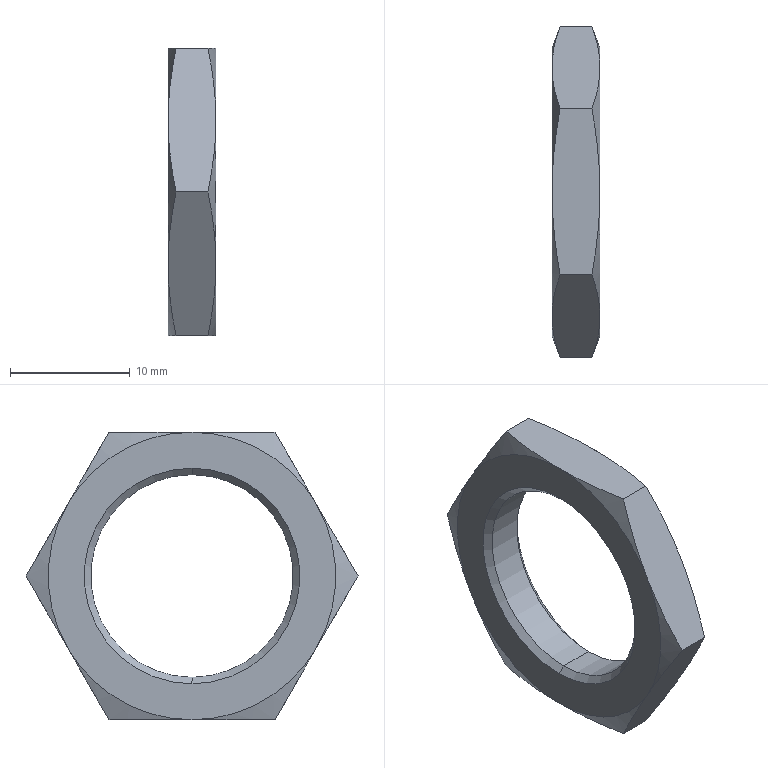Part | SolidWorks | features BaseBody 1 | 1 solid | 26 faces | box 4 x 27.713 x 24 mm | volume 1061 mm3 | cone 16 | plane 8 | cylinder 2 | commonest cylinder face diameters 16.917 x2
STEP:
#1=CARTESIAN_POINT('',(1.458,0.,8.459));
#2=VERTEX_POINT('',#1);
#3=CARTESIAN_POINT('',(1.458,0.,-8.459));
#4=VERTEX_POINT('',#3);
#5=CARTESIAN_POINT('',(1.458,0.,0.));
#6=DIRECTION('',(1.,0.,0.));
#7=DIRECTION('',(0.,0.,-1.));
#8=AXIS2_PLACEMENT_3D('',#5,#6,#7);
#9=CIRCLE('',#8,8.459);
#10=EDGE_CURVE('',#2,#4,#9,.T.);
#11=ORIENTED_EDGE('',*,*,#10,.F.);
#12=CARTESIAN_POINT('',(2.,0.,9.));
#13=VERTEX_POINT('',#12);
#14=CARTESIAN_POINT('',(2.,0.,9.));
#15=DIRECTION('',(0.7071,0.,0.7071));
#16=VECTOR('',#15,1000.);
#17=LINE('',#14,#16);
#18=EDGE_CURVE('',#2,#13,#17,.T.);
#19=ORIENTED_EDGE('',*,*,#18,.T.);
#20=CARTESIAN_POINT('',(2.,0.,-9.));
#21=VERTEX_POINT('',#20);
#22=CARTESIAN_POINT('',(2.,0.,0.));
#23=DIRECTION('',(1.,0.,0.));
#24=DIRECTION('',(0.,0.,-1.));
#25=AXIS2_PLACEMENT_3D('',#22,#23,#24);
#26=CIRCLE('',#25,9.);
#27=EDGE_CURVE('',#13,#21,#26,.T.);
#28=ORIENTED_EDGE('',*,*,#27,.T.);
#29=CARTESIAN_POINT('',(2.,0.,-9.));
#30=DIRECTION('',(0.7071,0.,-0.7071));
#31=VECTOR('',#30,1000.);
#32=LINE('',#29,#31);
#33=EDGE_CURVE('',#4,#21,#32,.T.);
#34=ORIENTED_EDGE('',*,*,#33,.F.);
#35=EDGE_LOOP('',(#11,#19,#28,#34));
#36=FACE_OUTER_BOUND('',#35,.T.);
#37=CARTESIAN_POINT('',(2.,0.,0.));
#38=DIRECTION('',(1.,0.,0.));
#39=DIRECTION('',(0.,0.,-1.));
#40=AXIS2_PLACEMENT_3D('',#37,#38,#39);
#41=CONICAL_SURFACE('',#40,9.,0.7854);
#42=ADVANCED_FACE('',(#36),#41,.F.);
#43=ORIENTED_EDGE('',*,*,#10,.T.);
#44=CARTESIAN_POINT('',(-1.458,0.,-8.459));
#45=VERTEX_POINT('',#44);
#46=CARTESIAN_POINT('',(2.,0.,-8.459));
#47=DIRECTION('',(-1.,0.,0.));
#48=VECTOR('',#47,1000.);
#49=LINE('',#46,#48);
#50=EDGE_CURVE('',#4,#45,#49,.T.);
#51=ORIENTED_EDGE('',*,*,#50,.T.);
#52=CARTESIAN_POINT('',(-1.458,0.,8.459));
#53=VERTEX_POINT('',#52);
#54=CARTESIAN_POINT('',(-1.458,0.,0.));
#55=DIRECTION('',(1.,0.,0.));
#56=DIRECTION('',(0.,0.,1.));
#57=AXIS2_PLACEMENT_3D('',#54,#55,#56);
#58=CIRCLE('',#57,8.459);
#59=EDGE_CURVE('',#53,#45,#58,.T.);
#60=ORIENTED_EDGE('',*,*,#59,.F.);
#61=CARTESIAN_POINT('',(2.,0.,8.459));
#62=DIRECTION('',(-1.,0.,0.));
#63=VECTOR('',#62,1000.);
#64=LINE('',#61,#63);
#65=EDGE_CURVE('',#2,#53,#64,.T.);
#66=ORIENTED_EDGE('',*,*,#65,.F.);
#67=EDGE_LOOP('',(#43,#51,#60,#66));
#68=FACE_OUTER_BOUND('',#67,.T.);
#69=CARTESIAN_POINT('',(2.,0.,0.));
#70=DIRECTION('',(-1.,0.,0.));
#71=DIRECTION('',(0.,0.,1.));
#72=AXIS2_PLACEMENT_3D('',#69,#70,#71);
#73=CYLINDRICAL_SURFACE('',#72,8.459);
#74=ADVANCED_FACE('',(#68),#73,.F.);
#75=ORIENTED_EDGE('',*,*,#59,.T.);
#76=CARTESIAN_POINT('',(-2.,0.,-9.));
#77=VERTEX_POINT('',#76);
#78=CARTESIAN_POINT('',(-2.,0.,-9.));
#79=DIRECTION('',(-0.7071,0.,-0.7071));
#80=VECTOR('',#79,1000.);
#81=LINE('',#78,#80);
#82=EDGE_CURVE('',#45,#77,#81,.T.);
#83=ORIENTED_EDGE('',*,*,#82,.T.);
#84=CARTESIAN_POINT('',(-2.,0.,9.));
#85=VERTEX_POINT('',#84);
#86=CARTESIAN_POINT('',(-2.,0.,0.));
#87=DIRECTION('',(1.,0.,0.));
#88=DIRECTION('',(0.,0.,1.));
#89=AXIS2_PLACEMENT_3D('',#86,#87,#88);
#90=CIRCLE('',#89,9.);
#91=EDGE_CURVE('',#85,#77,#90,.T.);
#92=ORIENTED_EDGE('',*,*,#91,.F.);
#93=CARTESIAN_POINT('',(-2.,0.,9.));
#94=DIRECTION('',(-0.7071,0.,0.7071));
#95=VECTOR('',#94,1000.);
#96=LINE('',#93,#95);
#97=EDGE_CURVE('',#53,#85,#96,.T.);
#98=ORIENTED_EDGE('',*,*,#97,.F.);
#99=EDGE_LOOP('',(#75,#83,#92,#98));
#100=FACE_OUTER_BOUND('',#99,.T.);
#101=CARTESIAN_POINT('',(-2.,0.,0.));
#102=DIRECTION('',(-1.,0.,0.));
#103=DIRECTION('',(0.,0.,1.));
#104=AXIS2_PLACEMENT_3D('',#101,#102,#103);
#105=CONICAL_SURFACE('',#104,9.,0.7854);
#106=ADVANCED_FACE('',(#100),#105,.F.);
#107=CARTESIAN_POINT('',(2.,10.392,6.));
#108=VERTEX_POINT('',#107);
#109=CARTESIAN_POINT('',(2.,10.392,-6.));
#110=VERTEX_POINT('',#109);
#111=CARTESIAN_POINT('',(2.,0.,0.));
#112=DIRECTION('',(-1.,0.,0.));
#113=DIRECTION('',(0.,0.,1.));
#114=AXIS2_PLACEMENT_3D('',#111,#112,#113);
#115=CIRCLE('',#114,12.);
#116=EDGE_CURVE('',#108,#110,#115,.T.);
#117=ORIENTED_EDGE('',*,*,#116,.F.);
#118=CARTESIAN_POINT('',(2.,0.,12.));
#119=VERTEX_POINT('',#118);
#120=CARTESIAN_POINT('',(2.,0.,0.));
#121=DIRECTION('',(-1.,0.,0.));
#122=DIRECTION('',(0.,0.,1.));
#123=AXIS2_PLACEMENT_3D('',#120,#121,#122);
#124=CIRCLE('',#123,12.);
#125=EDGE_CURVE('',#119,#108,#124,.T.);
#126=ORIENTED_EDGE('',*,*,#125,.F.);
#127=CARTESIAN_POINT('',(2.,-10.392,6.));
#128=VERTEX_POINT('',#127);
#129=CARTESIAN_POINT('',(2.,0.,0.));
#130=DIRECTION('',(-1.,0.,0.));
#131=DIRECTION('',(0.,0.,1.));
#132=AXIS2_PLACEMENT_3D('',#129,#130,#131);
#133=CIRCLE('',#132,12.);
#134=EDGE_CURVE('',#128,#119,#133,.T.);
#135=ORIENTED_EDGE('',*,*,#134,.F.);
#136=CARTESIAN_POINT('',(2.,-10.392,-6.));
#137=VERTEX_POINT('',#136);
#138=CARTESIAN_POINT('',(2.,0.,0.));
#139=DIRECTION('',(-1.,0.,0.));
#140=DIRECTION('',(0.,0.,1.));
#141=AXIS2_PLACEMENT_3D('',#138,#139,#140);
#142=CIRCLE('',#141,12.);
#143=EDGE_CURVE('',#137,#128,#142,.T.);
#144=ORIENTED_EDGE('',*,*,#143,.F.);
#145=CARTESIAN_POINT('',(2.,0.,-12.));
#146=VERTEX_POINT('',#145);
#147=CARTESIAN_POINT('',(2.,0.,0.));
#148=DIRECTION('',(-1.,0.,0.));
#149=DIRECTION('',(0.,0.,1.));
#150=AXIS2_PLACEMENT_3D('',#147,#148,#149);
#151=CIRCLE('',#150,12.);
#152=EDGE_CURVE('',#146,#137,#151,.T.);
#153=ORIENTED_EDGE('',*,*,#152,.F.);
#154=CARTESIAN_POINT('',(2.,0.,0.));
#155=DIRECTION('',(-1.,0.,0.));
#156=DIRECTION('',(0.,0.,1.));
#157=AXIS2_PLACEMENT_3D('',#154,#155,#156);
#158=CIRCLE('',#157,12.);
#159=EDGE_CURVE('',#110,#146,#158,.T.);
#160=ORIENTED_EDGE('',*,*,#159,.F.);
#161=EDGE_LOOP('',(#117,#126,#135,#144,#153,#160));
#162=FACE_OUTER_BOUND('',#161,.T.);
#163=CARTESIAN_POINT('',(2.,0.,0.));
#164=DIRECTION('',(1.,0.,0.));
#165=DIRECTION('',(0.,0.,-1.));
#166=AXIS2_PLACEMENT_3D('',#163,#164,#165);
#167=CIRCLE('',#166,9.);
#168=EDGE_CURVE('',#21,#13,#167,.T.);
#169=ORIENTED_EDGE('',*,*,#168,.F.);
#170=ORIENTED_EDGE('',*,*,#27,.F.);
#171=EDGE_LOOP('',(#169,#170));
#172=FACE_BOUND('',#171,.T.);
#173=CARTESIAN_POINT('',(2.,12.,0.));
#174=DIRECTION('',(-1.,0.,0.));
#175=DIRECTION('',(0.,0.,1.));
#176=AXIS2_PLACEMENT_3D('',#173,#174,#175);
#177=PLANE('',#176);
#178=ADVANCED_FACE('',(#162,#172),#177,.F.);
#179=CARTESIAN_POINT('',(1.324,6.928,-12.));
#180=VERTEX_POINT('',#179);
#181=CARTESIAN_POINT('',(1.324,6.928,-12.));
#182=CARTESIAN_POINT('',(1.533,7.501,-11.008));
#183=CARTESIAN_POINT('',(1.703,8.075,-10.013));
#184=CARTESIAN_POINT('',(1.937,9.23,-8.014));
#185=CARTESIAN_POINT('',(2.,9.809,-7.01));
#186=CARTESIAN_POINT('',(2.,10.392,-6.));
#187=B_SPLINE_CURVE_WITH_KNOTS('',3,(#181,#182,#183,#184,#185,#186),.UNSPECIFIED.,.F.,.F.,(4,2,4),(0.,0.003481,0.006961),.UNSPECIFIED.);
#188=EDGE_CURVE('',#180,#110,#187,.T.);
#189=ORIENTED_EDGE('',*,*,#188,.T.);
#190=ORIENTED_EDGE('',*,*,#159,.T.);
#191=CARTESIAN_POINT('',(2.,0.,-12.));
#192=CARTESIAN_POINT('',(2.,1.166,-12.));
#193=CARTESIAN_POINT('',(1.937,2.325,-12.));
#194=CARTESIAN_POINT('',(1.703,4.634,-12.));
#195=CARTESIAN_POINT('',(1.533,5.783,-12.));
#196=CARTESIAN_POINT('',(1.324,6.928,-12.));
#197=B_SPLINE_CURVE_WITH_KNOTS('',3,(#191,#192,#193,#194,#195,#196),.UNSPECIFIED.,.F.,.F.,(4,2,4),(0.,0.003481,0.006961),.UNSPECIFIED.);
#198=EDGE_CURVE('',#146,#180,#197,.T.);
#199=ORIENTED_EDGE('',*,*,#198,.T.);
#200=EDGE_LOOP('',(#189,#190,#199));
#201=FACE_OUTER_BOUND('',#200,.T.);
#202=CARTESIAN_POINT('',(1.32,0.,0.));
#203=DIRECTION('',(-1.,0.,0.));
#204=DIRECTION('',(0.,0.,1.));
#205=AXIS2_PLACEMENT_3D('',#202,#203,#204);
#206=CONICAL_SURFACE('',#205,13.868,1.222);
#207=ADVANCED_FACE('',(#201),#206,.T.);
#208=CARTESIAN_POINT('',(1.324,13.856,-0.000000041));
#209=VERTEX_POINT('',#208);
#210=CARTESIAN_POINT('',(2.,10.392,-6.));
#211=CARTESIAN_POINT('',(2.,10.975,-4.99));
#212=CARTESIAN_POINT('',(1.937,11.555,-3.986));
#213=CARTESIAN_POINT('',(1.703,12.709,-1.987));
#214=CARTESIAN_POINT('',(1.533,13.284,-0.9919));
#215=CARTESIAN_POINT('',(1.324,13.856,-0.000000041));
#216=B_SPLINE_CURVE_WITH_KNOTS('',3,(#210,#211,#212,#213,#214,#215),.UNSPECIFIED.,.F.,.F.,(4,2,4),(0.,0.003481,0.006961),.UNSPECIFIED.);
#217=EDGE_CURVE('',#110,#209,#216,.T.);
#218=ORIENTED_EDGE('',*,*,#217,.T.);
#219=CARTESIAN_POINT('',(1.324,13.856,-0.000000041));
#220=CARTESIAN_POINT('',(1.533,13.284,0.9919));
#221=CARTESIAN_POINT('',(1.703,12.709,1.987));
#222=CARTESIAN_POINT('',(1.937,11.555,3.986));
#223=CARTESIAN_POINT('',(2.,10.975,4.99));
#224=CARTESIAN_POINT('',(2.,10.392,6.));
#225=B_SPLINE_CURVE_WITH_KNOTS('',3,(#219,#220,#221,#222,#223,#224),.UNSPECIFIED.,.F.,.F.,(4,2,4),(0.,0.003481,0.006961),.UNSPECIFIED.);
#226=EDGE_CURVE('',#209,#108,#225,.T.);
#227=ORIENTED_EDGE('',*,*,#226,.T.);
#228=ORIENTED_EDGE('',*,*,#116,.T.);
#229=EDGE_LOOP('',(#218,#227,#228));
#230=FACE_OUTER_BOUND('',#229,.T.);
#231=CARTESIAN_POINT('',(1.32,0.,0.));
#232=DIRECTION('',(-1.,0.,0.));
#233=DIRECTION('',(0.,0.,1.));
#234=AXIS2_PLACEMENT_3D('',#231,#232,#233);
#235=CONICAL_SURFACE('',#234,13.868,1.222);
#236=ADVANCED_FACE('',(#230),#235,.T.);
#237=CARTESIAN_POINT('',(1.324,6.928,12.));
#238=VERTEX_POINT('',#237);
#239=CARTESIAN_POINT('',(2.,10.392,6.));
#240=CARTESIAN_POINT('',(2.,9.809,7.01));
#241=CARTESIAN_POINT('',(1.937,9.23,8.014));
#242=CARTESIAN_POINT('',(1.703,8.075,10.013));
#243=CARTESIAN_POINT('',(1.533,7.501,11.008));
#244=CARTESIAN_POINT('',(1.324,6.928,12.));
#245=B_SPLINE_CURVE_WITH_KNOTS('',3,(#239,#240,#241,#242,#243,#244),.UNSPECIFIED.,.F.,.F.,(4,2,4),(0.,0.003481,0.006961),.UNSPECIFIED.);
#246=EDGE_CURVE('',#108,#238,#245,.T.);
#247=ORIENTED_EDGE('',*,*,#246,.T.);
#248=CARTESIAN_POINT('',(1.324,6.928,12.));
#249=CARTESIAN_POINT('',(1.533,5.783,12.));
#250=CARTESIAN_POINT('',(1.703,4.634,12.));
#251=CARTESIAN_POINT('',(1.937,2.325,12.));
#252=CARTESIAN_POINT('',(2.,1.166,12.));
#253=CARTESIAN_POINT('',(2.,0.,12.));
#254=B_SPLINE_CURVE_WITH_KNOTS('',3,(#248,#249,#250,#251,#252,#253),.UNSPECIFIED.,.F.,.F.,(4,2,4),(0.,0.003481,0.006961),.UNSPECIFIED.);
#255=EDGE_CURVE('',#238,#119,#254,.T.);
#256=ORIENTED_EDGE('',*,*,#255,.T.);
#257=ORIENTED_EDGE('',*,*,#125,.T.);
#258=EDGE_LOOP('',(#247,#256,#257));
#259=FACE_OUTER_BOUND('',#258,.T.);
#260=CARTESIAN_POINT('',(1.32,0.,0.));
#261=DIRECTION('',(-1.,0.,0.));
#262=DIRECTION('',(0.,0.,1.));
#263=AXIS2_PLACEMENT_3D('',#260,#261,#262);
#264=CONICAL_SURFACE('',#263,13.868,1.222);
#265=ADVANCED_FACE('',(#259),#264,.T.);
#266=CARTESIAN_POINT('',(1.324,-6.928,12.));
#267=VERTEX_POINT('',#266);
#268=CARTESIAN_POINT('',(2.,0.,12.));
#269=CARTESIAN_POINT('',(2.,-1.166,12.));
#270=CARTESIAN_POINT('',(1.937,-2.325,12.));
#271=CARTESIAN_POINT('',(1.703,-4.634,12.));
#272=CARTESIAN_POINT('',(1.533,-5.783,12.));
#273=CARTESIAN_POINT('',(1.324,-6.928,12.));
#274=B_SPLINE_CURVE_WITH_KNOTS('',3,(#268,#269,#270,#271,#272,#273),.UNSPECIFIED.,.F.,.F.,(4,2,4),(0.,0.003481,0.006961),.UNSPECIFIED.);
#275=EDGE_CURVE('',#119,#267,#274,.T.);
#276=ORIENTED_EDGE('',*,*,#275,.T.);
#277=CARTESIAN_POINT('',(1.324,-6.928,12.));
#278=CARTESIAN_POINT('',(1.533,-7.501,11.008));
#279=CARTESIAN_POINT('',(1.703,-8.075,10.013));
#280=CARTESIAN_POINT('',(1.937,-9.23,8.014));
#281=CARTESIAN_POINT('',(2.,-9.809,7.01));
#282=CARTESIAN_POINT('',(2.,-10.392,6.));
#283=B_SPLINE_CURVE_WITH_KNOTS('',3,(#277,#278,#279,#280,#281,#282),.UNSPECIFIED.,.F.,.F.,(4,2,4),(0.,0.003481,0.006961),.UNSPECIFIED.);
#284=EDGE_CURVE('',#267,#128,#283,.T.);
#285=ORIENTED_EDGE('',*,*,#284,.T.);
#286=ORIENTED_EDGE('',*,*,#134,.T.);
#287=EDGE_LOOP('',(#276,#285,#286));
#288=FACE_OUTER_BOUND('',#287,.T.);
#289=CARTESIAN_POINT('',(1.32,0.,0.));
#290=DIRECTION('',(-1.,0.,0.));
#291=DIRECTION('',(0.,0.,1.));
#292=AXIS2_PLACEMENT_3D('',#289,#290,#291);
#293=CONICAL_SURFACE('',#292,13.868,1.222);
#294=ADVANCED_FACE('',(#288),#293,.T.);
#295=CARTESIAN_POINT('',(1.324,-13.856,0.000000041));
#296=VERTEX_POINT('',#295);
#297=CARTESIAN_POINT('',(1.324,-13.856,0.000000041));
#298=CARTESIAN_POINT('',(1.533,-13.284,-0.9919));
#299=CARTESIAN_POINT('',(1.703,-12.709,-1.987));
#300=CARTESIAN_POINT('',(1.937,-11.555,-3.986));
#301=CARTESIAN_POINT('',(2.,-10.975,-4.99));
#302=CARTESIAN_POINT('',(2.,-10.392,-6.));
#303=B_SPLINE_CURVE_WITH_KNOTS('',3,(#297,#298,#299,#300,#301,#302),.UNSPECIFIED.,.F.,.F.,(4,2,4),(0.,0.003481,0.006961),.UNSPECIFIED.);
#304=EDGE_CURVE('',#296,#137,#303,.T.);
#305=ORIENTED_EDGE('',*,*,#304,.T.);
#306=ORIENTED_EDGE('',*,*,#143,.T.);
#307=CARTESIAN_POINT('',(2.,-10.392,6.));
#308=CARTESIAN_POINT('',(2.,-10.975,4.99));
#309=CARTESIAN_POINT('',(1.937,-11.555,3.986));
#310=CARTESIAN_POINT('',(1.703,-12.709,1.987));
#311=CARTESIAN_POINT('',(1.533,-13.284,0.9919));
#312=CARTESIAN_POINT('',(1.324,-13.856,0.000000041));
#313=B_SPLINE_CURVE_WITH_KNOTS('',3,(#307,#308,#309,#310,#311,#312),.UNSPECIFIED.,.F.,.F.,(4,2,4),(0.,0.003481,0.006961),.UNSPECIFIED.);
#314=EDGE_CURVE('',#128,#296,#313,.T.);
#315=ORIENTED_EDGE('',*,*,#314,.T.);
#316=EDGE_LOOP('',(#305,#306,#315));
#317=FACE_OUTER_BOUND('',#316,.T.);
#318=CARTESIAN_POINT('',(1.32,0.,0.));
#319=DIRECTION('',(-1.,0.,0.));
#320=DIRECTION('',(0.,0.,1.));
#321=AXIS2_PLACEMENT_3D('',#318,#319,#320);
#322=CONICAL_SURFACE('',#321,13.868,1.222);
#323=ADVANCED_FACE('',(#317),#322,.T.);
#324=CARTESIAN_POINT('',(1.324,-6.928,-12.));
#325=VERTEX_POINT('',#324);
#326=CARTESIAN_POINT('',(1.324,-6.928,-12.));
#327=CARTESIAN_POINT('',(1.533,-5.783,-12.));
#328=CARTESIAN_POINT('',(1.703,-4.634,-12.));
#329=CARTESIAN_POINT('',(1.937,-2.325,-12.));
#330=CARTESIAN_POINT('',(2.,-1.166,-12.));
#331=CARTESIAN_POINT('',(2.,0.,-12.));
#332=B_SPLINE_CURVE_WITH_KNOTS('',3,(#326,#327,#328,#329,#330,#331),.UNSPECIFIED.,.F.,.F.,(4,2,4),(0.,0.003481,0.006961),.UNSPECIFIED.);
#333=EDGE_CURVE('',#325,#146,#332,.T.);
#334=ORIENTED_EDGE('',*,*,#333,.T.);
#335=ORIENTED_EDGE('',*,*,#152,.T.);
#336=CARTESIAN_POINT('',(2.,-10.392,-6.));
#337=CARTESIAN_POINT('',(2.,-9.809,-7.01));
#338=CARTESIAN_POINT('',(1.937,-9.23,-8.014));
#339=CARTESIAN_POINT('',(1.703,-8.075,-10.013));
#340=CARTESIAN_POINT('',(1.533,-7.501,-11.008));
#341=CARTESIAN_POINT('',(1.324,-6.928,-12.));
#342=B_SPLINE_CURVE_WITH_KNOTS('',3,(#336,#337,#338,#339,#340,#341),.UNSPECIFIED.,.F.,.F.,(4,2,4),(0.,0.003481,0.006961),.UNSPECIFIED.);
#343=EDGE_CURVE('',#137,#325,#342,.T.);
#344=ORIENTED_EDGE('',*,*,#343,.T.);
#345=EDGE_LOOP('',(#334,#335,#344));
#346=FACE_OUTER_BOUND('',#345,.T.);
#347=CARTESIAN_POINT('',(1.32,0.,0.));
#348=DIRECTION('',(-1.,0.,0.));
#349=DIRECTION('',(0.,0.,1.));
#350=AXIS2_PLACEMENT_3D('',#347,#348,#349);
#351=CONICAL_SURFACE('',#350,13.868,1.222);
#352=ADVANCED_FACE('',(#346),#351,.T.);
#353=ORIENTED_EDGE('',*,*,#18,.F.);
#354=CARTESIAN_POINT('',(1.458,0.,0.));
#355=DIRECTION('',(1.,0.,0.));
#356=DIRECTION('',(0.,0.,-1.));
#357=AXIS2_PLACEMENT_3D('',#354,#355,#356);
#358=CIRCLE('',#357,8.459);
#359=EDGE_CURVE('',#4,#2,#358,.T.);
#360=ORIENTED_EDGE('',*,*,#359,.F.);
#361=ORIENTED_EDGE('',*,*,#33,.T.);
#362=ORIENTED_EDGE('',*,*,#168,.T.);
#363=EDGE_LOOP('',(#353,#360,#361,#362));
#364=FACE_OUTER_BOUND('',#363,.T.);
#365=CARTESIAN_POINT('',(2.,0.,0.));
#366=DIRECTION('',(1.,0.,0.));
#367=DIRECTION('',(0.,0.,-1.));
#368=AXIS2_PLACEMENT_3D('',#365,#366,#367);
#369=CONICAL_SURFACE('',#368,9.,0.7854);
#370=ADVANCED_FACE('',(#364),#369,.F.);
#371=ORIENTED_EDGE('',*,*,#217,.F.);
#372=ORIENTED_EDGE('',*,*,#188,.F.);
#373=CARTESIAN_POINT('',(-1.324,6.928,-12.));
#374=VERTEX_POINT('',#373);
#375=CARTESIAN_POINT('',(4.,6.928,-12.));
#376=DIRECTION('',(1.,0.,0.));
#377=VECTOR('',#376,1000.);
#378=LINE('',#375,#377);
#379=EDGE_CURVE('',#374,#180,#378,.T.);
#380=ORIENTED_EDGE('',*,*,#379,.F.);
#381=CARTESIAN_POINT('',(-2.,10.392,-6.));
#382=VERTEX_POINT('',#381);
#383=CARTESIAN_POINT('',(-2.,10.392,-6.));
#384=CARTESIAN_POINT('',(-2.,9.809,-7.01));
#385=CARTESIAN_POINT('',(-1.937,9.23,-8.014));
#386=CARTESIAN_POINT('',(-1.703,8.075,-10.013));
#387=CARTESIAN_POINT('',(-1.533,7.501,-11.008));
#388=CARTESIAN_POINT('',(-1.324,6.928,-12.));
#389=B_SPLINE_CURVE_WITH_KNOTS('',3,(#383,#384,#385,#386,#387,#388),.UNSPECIFIED.,.F.,.F.,(4,2,4),(0.,0.003481,0.006961),.UNSPECIFIED.);
#390=EDGE_CURVE('',#382,#374,#389,.T.);
#391=ORIENTED_EDGE('',*,*,#390,.F.);
#392=CARTESIAN_POINT('',(-1.324,13.856,0.));
#393=VERTEX_POINT('',#392);
#394=CARTESIAN_POINT('',(-1.324,13.856,0.));
#395=CARTESIAN_POINT('',(-1.533,13.284,-0.9919));
#396=CARTESIAN_POINT('',(-1.703,12.709,-1.987));
#397=CARTESIAN_POINT('',(-1.937,11.555,-3.986));
#398=CARTESIAN_POINT('',(-2.,10.975,-4.99));
#399=CARTESIAN_POINT('',(-2.,10.392,-6.));
#400=B_SPLINE_CURVE_WITH_KNOTS('',3,(#394,#395,#396,#397,#398,#399),.UNSPECIFIED.,.F.,.F.,(4,2,4),(0.,0.003481,0.006961),.UNSPECIFIED.);
#401=EDGE_CURVE('',#393,#382,#400,.T.);
#402=ORIENTED_EDGE('',*,*,#401,.F.);
#403=CARTESIAN_POINT('',(4.,13.856,0.));
#404=DIRECTION('',(-1.,0.,0.));
#405=VECTOR('',#404,1000.);
#406=LINE('',#403,#405);
#407=EDGE_CURVE('',#209,#393,#406,.T.);
#408=ORIENTED_EDGE('',*,*,#407,.F.);
#409=EDGE_LOOP('',(#371,#372,#380,#391,#402,#408));
#410=FACE_OUTER_BOUND('',#409,.T.);
#411=CARTESIAN_POINT('',(4.,6.928,-12.));
#412=DIRECTION('',(0.,-0.866,0.5));
#413=DIRECTION('',(0.,-0.5,-0.866));
#414=AXIS2_PLACEMENT_3D('',#411,#412,#413);
#415=PLANE('',#414);
#416=ADVANCED_FACE('',(#410),#415,.F.);
#417=ORIENTED_EDGE('',*,*,#198,.F.);
#418=ORIENTED_EDGE('',*,*,#333,.F.);
#419=CARTESIAN_POINT('',(-1.324,-6.928,-12.));
#420=VERTEX_POINT('',#419);
#421=CARTESIAN_POINT('',(4.,-6.928,-12.));
#422=DIRECTION('',(1.,0.,0.));
#423=VECTOR('',#422,1000.);
#424=LINE('',#421,#423);
#425=EDGE_CURVE('',#420,#325,#424,.T.);
#426=ORIENTED_EDGE('',*,*,#425,.F.);
#427=CARTESIAN_POINT('',(-2.,0.,-12.));
#428=VERTEX_POINT('',#427);
#429=CARTESIAN_POINT('',(-2.,0.,-12.));
#430=CARTESIAN_POINT('',(-2.,-1.166,-12.));
#431=CARTESIAN_POINT('',(-1.937,-2.325,-12.));
#432=CARTESIAN_POINT('',(-1.703,-4.634,-12.));
#433=CARTESIAN_POINT('',(-1.533,-5.783,-12.));
#434=CARTESIAN_POINT('',(-1.324,-6.928,-12.));
#435=B_SPLINE_CURVE_WITH_KNOTS('',3,(#429,#430,#431,#432,#433,#434),.UNSPECIFIED.,.F.,.F.,(4,2,4),(0.,0.003481,0.006961),.UNSPECIFIED.);
#436=EDGE_CURVE('',#428,#420,#435,.T.);
#437=ORIENTED_EDGE('',*,*,#436,.F.);
#438=CARTESIAN_POINT('',(-1.324,6.928,-12.));
#439=CARTESIAN_POINT('',(-1.533,5.783,-12.));
#440=CARTESIAN_POINT('',(-1.703,4.634,-12.));
#441=CARTESIAN_POINT('',(-1.937,2.325,-12.));
#442=CARTESIAN_POINT('',(-2.,1.166,-12.));
#443=CARTESIAN_POINT('',(-2.,0.,-12.));
#444=B_SPLINE_CURVE_WITH_KNOTS('',3,(#438,#439,#440,#441,#442,#443),.UNSPECIFIED.,.F.,.F.,(4,2,4),(0.,0.003481,0.006961),.UNSPECIFIED.);
#445=EDGE_CURVE('',#374,#428,#444,.T.);
#446=ORIENTED_EDGE('',*,*,#445,.F.);
#447=ORIENTED_EDGE('',*,*,#379,.T.);
#448=EDGE_LOOP('',(#417,#418,#426,#437,#446,#447));
#449=FACE_OUTER_BOUND('',#448,.T.);
#450=CARTESIAN_POINT('',(4.,-6.928,-12.));
#451=DIRECTION('',(0.,0.,1.));
#452=DIRECTION('',(1.,0.,0.));
#453=AXIS2_PLACEMENT_3D('',#450,#451,#452);
#454=PLANE('',#453);
#455=ADVANCED_FACE('',(#449),#454,.F.);
#456=ORIENTED_EDGE('',*,*,#246,.F.);
#457=ORIENTED_EDGE('',*,*,#226,.F.);
#458=ORIENTED_EDGE('',*,*,#407,.T.);
#459=CARTESIAN_POINT('',(-2.,10.392,6.));
#460=VERTEX_POINT('',#459);
#461=CARTESIAN_POINT('',(-2.,10.392,6.));
#462=CARTESIAN_POINT('',(-2.,10.975,4.99));
#463=CARTESIAN_POINT('',(-1.937,11.555,3.986));
#464=CARTESIAN_POINT('',(-1.703,12.709,1.987));
#465=CARTESIAN_POINT('',(-1.533,13.284,0.9919));
#466=CARTESIAN_POINT('',(-1.324,13.856,0.));
#467=B_SPLINE_CURVE_WITH_KNOTS('',3,(#461,#462,#463,#464,#465,#466),.UNSPECIFIED.,.F.,.F.,(4,2,4),(0.,0.003481,0.006961),.UNSPECIFIED.);
#468=EDGE_CURVE('',#460,#393,#467,.T.);
#469=ORIENTED_EDGE('',*,*,#468,.F.);
#470=CARTESIAN_POINT('',(-1.324,6.928,12.));
#471=VERTEX_POINT('',#470);
#472=CARTESIAN_POINT('',(-1.324,6.928,12.));
#473=CARTESIAN_POINT('',(-1.533,7.501,11.008));
#474=CARTESIAN_POINT('',(-1.703,8.075,10.013));
#475=CARTESIAN_POINT('',(-1.937,9.23,8.014));
#476=CARTESIAN_POINT('',(-2.,9.809,7.01));
#477=CARTESIAN_POINT('',(-2.,10.392,6.));
#478=B_SPLINE_CURVE_WITH_KNOTS('',3,(#472,#473,#474,#475,#476,#477),.UNSPECIFIED.,.F.,.F.,(4,2,4),(0.,0.003481,0.006961),.UNSPECIFIED.);
#479=EDGE_CURVE('',#471,#460,#478,.T.);
#480=ORIENTED_EDGE('',*,*,#479,.F.);
#481=CARTESIAN_POINT('',(4.,6.928,12.));
#482=DIRECTION('',(-1.,0.,0.));
#483=VECTOR('',#482,1000.);
#484=LINE('',#481,#483);
#485=EDGE_CURVE('',#238,#471,#484,.T.);
#486=ORIENTED_EDGE('',*,*,#485,.F.);
#487=EDGE_LOOP('',(#456,#457,#458,#469,#480,#486));
#488=FACE_OUTER_BOUND('',#487,.T.);
#489=CARTESIAN_POINT('',(4.,13.856,0.));
#490=DIRECTION('',(0.,-0.866,-0.5));
#491=DIRECTION('',(0.,0.5,-0.866));
#492=AXIS2_PLACEMENT_3D('',#489,#490,#491);
#493=PLANE('',#492);
#494=ADVANCED_FACE('',(#488),#493,.F.);
#495=ORIENTED_EDGE('',*,*,#275,.F.);
#496=ORIENTED_EDGE('',*,*,#255,.F.);
#497=ORIENTED_EDGE('',*,*,#485,.T.);
#498=CARTESIAN_POINT('',(-2.,0.,12.));
#499=VERTEX_POINT('',#498);
#500=CARTESIAN_POINT('',(-2.,0.,12.));
#501=CARTESIAN_POINT('',(-2.,1.166,12.));
#502=CARTESIAN_POINT('',(-1.937,2.325,12.));
#503=CARTESIAN_POINT('',(-1.703,4.634,12.));
#504=CARTESIAN_POINT('',(-1.533,5.783,12.));
#505=CARTESIAN_POINT('',(-1.324,6.928,12.));
#506=B_SPLINE_CURVE_WITH_KNOTS('',3,(#500,#501,#502,#503,#504,#505),.UNSPECIFIED.,.F.,.F.,(4,2,4),(0.,0.003481,0.006961),.UNSPECIFIED.);
#507=EDGE_CURVE('',#499,#471,#506,.T.);
#508=ORIENTED_EDGE('',*,*,#507,.F.);
#509=CARTESIAN_POINT('',(-1.324,-6.928,12.));
#510=VERTEX_POINT('',#509);
#511=CARTESIAN_POINT('',(-1.324,-6.928,12.));
#512=CARTESIAN_POINT('',(-1.533,-5.783,12.));
#513=CARTESIAN_POINT('',(-1.703,-4.634,12.));
#514=CARTESIAN_POINT('',(-1.937,-2.325,12.));
#515=CARTESIAN_POINT('',(-2.,-1.166,12.));
#516=CARTESIAN_POINT('',(-2.,0.,12.));
#517=B_SPLINE_CURVE_WITH_KNOTS('',3,(#511,#512,#513,#514,#515,#516),.UNSPECIFIED.,.F.,.F.,(4,2,4),(0.,0.003481,0.006961),.UNSPECIFIED.);
#518=EDGE_CURVE('',#510,#499,#517,.T.);
#519=ORIENTED_EDGE('',*,*,#518,.F.);
#520=CARTESIAN_POINT('',(4.,-6.928,12.));
#521=DIRECTION('',(-1.,0.,0.));
#522=VECTOR('',#521,1000.);
#523=LINE('',#520,#522);
#524=EDGE_CURVE('',#267,#510,#523,.T.);
#525=ORIENTED_EDGE('',*,*,#524,.F.);
#526=EDGE_LOOP('',(#495,#496,#497,#508,#519,#525));
#527=FACE_OUTER_BOUND('',#526,.T.);
#528=CARTESIAN_POINT('',(4.,6.928,12.));
#529=DIRECTION('',(0.,0.,-1.));
#530=DIRECTION('',(-1.,0.,0.));
#531=AXIS2_PLACEMENT_3D('',#528,#529,#530);
#532=PLANE('',#531);
#533=ADVANCED_FACE('',(#527),#532,.F.);
#534=ORIENTED_EDGE('',*,*,#314,.F.);
#535=ORIENTED_EDGE('',*,*,#284,.F.);
#536=ORIENTED_EDGE('',*,*,#524,.T.);
#537=CARTESIAN_POINT('',(-2.,-10.392,6.));
#538=VERTEX_POINT('',#537);
#539=CARTESIAN_POINT('',(-2.,-10.392,6.));
#540=CARTESIAN_POINT('',(-2.,-9.809,7.01));
#541=CARTESIAN_POINT('',(-1.937,-9.23,8.014));
#542=CARTESIAN_POINT('',(-1.703,-8.075,10.013));
#543=CARTESIAN_POINT('',(-1.533,-7.501,11.008));
#544=CARTESIAN_POINT('',(-1.324,-6.928,12.));
#545=B_SPLINE_CURVE_WITH_KNOTS('',3,(#539,#540,#541,#542,#543,#544),.UNSPECIFIED.,.F.,.F.,(4,2,4),(0.,0.003481,0.006961),.UNSPECIFIED.);
#546=EDGE_CURVE('',#538,#510,#545,.T.);
#547=ORIENTED_EDGE('',*,*,#546,.F.);
#548=CARTESIAN_POINT('',(-1.324,-13.856,0.));
#549=VERTEX_POINT('',#548);
#550=CARTESIAN_POINT('',(-1.324,-13.856,0.));
#551=CARTESIAN_POINT('',(-1.533,-13.284,0.9919));
#552=CARTESIAN_POINT('',(-1.703,-12.709,1.987));
#553=CARTESIAN_POINT('',(-1.937,-11.555,3.986));
#554=CARTESIAN_POINT('',(-2.,-10.975,4.99));
#555=CARTESIAN_POINT('',(-2.,-10.392,6.));
#556=B_SPLINE_CURVE_WITH_KNOTS('',3,(#550,#551,#552,#553,#554,#555),.UNSPECIFIED.,.F.,.F.,(4,2,4),(0.,0.003481,0.006961),.UNSPECIFIED.);
#557=EDGE_CURVE('',#549,#538,#556,.T.);
#558=ORIENTED_EDGE('',*,*,#557,.F.);
#559=CARTESIAN_POINT('',(4.,-13.856,0.));
#560=DIRECTION('',(-1.,0.,0.));
#561=VECTOR('',#560,1000.);
#562=LINE('',#559,#561);
#563=EDGE_CURVE('',#296,#549,#562,.T.);
#564=ORIENTED_EDGE('',*,*,#563,.F.);
#565=EDGE_LOOP('',(#534,#535,#536,#547,#558,#564));
#566=FACE_OUTER_BOUND('',#565,.T.);
#567=CARTESIAN_POINT('',(4.,-6.928,12.));
#568=DIRECTION('',(0.,0.866,-0.5));
#569=DIRECTION('',(0.,0.5,0.866));
#570=AXIS2_PLACEMENT_3D('',#567,#568,#569);
#571=PLANE('',#570);
#572=ADVANCED_FACE('',(#566),#571,.F.);
#573=ORIENTED_EDGE('',*,*,#343,.F.);
#574=ORIENTED_EDGE('',*,*,#304,.F.);
#575=ORIENTED_EDGE('',*,*,#563,.T.);
#576=CARTESIAN_POINT('',(-2.,-10.392,-6.));
#577=VERTEX_POINT('',#576);
#578=CARTESIAN_POINT('',(-2.,-10.392,-6.));
#579=CARTESIAN_POINT('',(-2.,-10.975,-4.99));
#580=CARTESIAN_POINT('',(-1.937,-11.555,-3.986));
#581=CARTESIAN_POINT('',(-1.703,-12.709,-1.987));
#582=CARTESIAN_POINT('',(-1.533,-13.284,-0.9919));
#583=CARTESIAN_POINT('',(-1.324,-13.856,0.));
#584=B_SPLINE_CURVE_WITH_KNOTS('',3,(#578,#579,#580,#581,#582,#583),.UNSPECIFIED.,.F.,.F.,(4,2,4),(0.,0.003481,0.006961),.UNSPECIFIED.);
#585=EDGE_CURVE('',#577,#549,#584,.T.);
#586=ORIENTED_EDGE('',*,*,#585,.F.);
#587=CARTESIAN_POINT('',(-1.324,-6.928,-12.));
#588=CARTESIAN_POINT('',(-1.533,-7.501,-11.008));
#589=CARTESIAN_POINT('',(-1.703,-8.075,-10.013));
#590=CARTESIAN_POINT('',(-1.937,-9.23,-8.014));
#591=CARTESIAN_POINT('',(-2.,-9.809,-7.01));
#592=CARTESIAN_POINT('',(-2.,-10.392,-6.));
#593=B_SPLINE_CURVE_WITH_KNOTS('',3,(#587,#588,#589,#590,#591,#592),.UNSPECIFIED.,.F.,.F.,(4,2,4),(0.,0.003481,0.006961),.UNSPECIFIED.);
#594=EDGE_CURVE('',#420,#577,#593,.T.);
#595=ORIENTED_EDGE('',*,*,#594,.F.);
#596=ORIENTED_EDGE('',*,*,#425,.T.);
#597=EDGE_LOOP('',(#573,#574,#575,#586,#595,#596));
#598=FACE_OUTER_BOUND('',#597,.T.);
#599=CARTESIAN_POINT('',(4.,-13.856,0.));
#600=DIRECTION('',(0.,0.866,0.5));
#601=DIRECTION('',(0.,-0.5,0.866));
#602=AXIS2_PLACEMENT_3D('',#599,#600,#601);
#603=PLANE('',#602);
#604=ADVANCED_FACE('',(#598),#603,.F.);
#605=ORIENTED_EDGE('',*,*,#50,.F.);
#606=ORIENTED_EDGE('',*,*,#359,.T.);
#607=ORIENTED_EDGE('',*,*,#65,.T.);
#608=CARTESIAN_POINT('',(-1.458,0.,0.));
#609=DIRECTION('',(1.,0.,0.));
#610=DIRECTION('',(0.,0.,1.));
#611=AXIS2_PLACEMENT_3D('',#608,#609,#610);
#612=CIRCLE('',#611,8.459);
#613=EDGE_CURVE('',#45,#53,#612,.T.);
#614=ORIENTED_EDGE('',*,*,#613,.F.);
#615=EDGE_LOOP('',(#605,#606,#607,#614));
#616=FACE_OUTER_BOUND('',#615,.T.);
#617=CARTESIAN_POINT('',(2.,0.,0.));
#618=DIRECTION('',(-1.,0.,0.));
#619=DIRECTION('',(0.,0.,1.));
#620=AXIS2_PLACEMENT_3D('',#617,#618,#619);
#621=CYLINDRICAL_SURFACE('',#620,8.459);
#622=ADVANCED_FACE('',(#616),#621,.F.);
#623=ORIENTED_EDGE('',*,*,#390,.T.);
#624=ORIENTED_EDGE('',*,*,#445,.T.);
#625=CARTESIAN_POINT('',(-2.,0.,0.));
#626=DIRECTION('',(1.,0.,0.));
#627=DIRECTION('',(0.,0.,-1.));
#628=AXIS2_PLACEMENT_3D('',#625,#626,#627);
#629=CIRCLE('',#628,12.);
#630=EDGE_CURVE('',#428,#382,#629,.T.);
#631=ORIENTED_EDGE('',*,*,#630,.T.);
#632=EDGE_LOOP('',(#623,#624,#631));
#633=FACE_OUTER_BOUND('',#632,.T.);
#634=CARTESIAN_POINT('',(-1.32,0.,0.));
#635=DIRECTION('',(1.,0.,0.));
#636=DIRECTION('',(0.,0.,-1.));
#637=AXIS2_PLACEMENT_3D('',#634,#635,#636);
#638=CONICAL_SURFACE('',#637,13.868,1.222);
#639=ADVANCED_FACE('',(#633),#638,.T.);
#640=CARTESIAN_POINT('',(-2.,0.,0.));
#641=DIRECTION('',(1.,0.,0.));
#642=DIRECTION('',(0.,0.,-1.));
#643=AXIS2_PLACEMENT_3D('',#640,#641,#642);
#644=CIRCLE('',#643,12.);
#645=EDGE_CURVE('',#382,#460,#644,.T.);
#646=ORIENTED_EDGE('',*,*,#645,.T.);
#647=ORIENTED_EDGE('',*,*,#468,.T.);
#648=ORIENTED_EDGE('',*,*,#401,.T.);
#649=EDGE_LOOP('',(#646,#647,#648));
#650=FACE_OUTER_BOUND('',#649,.T.);
#651=CARTESIAN_POINT('',(-1.32,0.,0.));
#652=DIRECTION('',(1.,0.,0.));
#653=DIRECTION('',(0.,0.,-1.));
#654=AXIS2_PLACEMENT_3D('',#651,#652,#653);
#655=CONICAL_SURFACE('',#654,13.868,1.222);
#656=ADVANCED_FACE('',(#650),#655,.T.);
#657=ORIENTED_EDGE('',*,*,#436,.T.);
#658=ORIENTED_EDGE('',*,*,#594,.T.);
#659=CARTESIAN_POINT('',(-2.,0.,0.));
#660=DIRECTION('',(1.,0.,0.));
#661=DIRECTION('',(0.,0.,-1.));
#662=AXIS2_PLACEMENT_3D('',#659,#660,#661);
#663=CIRCLE('',#662,12.);
#664=EDGE_CURVE('',#577,#428,#663,.T.);
#665=ORIENTED_EDGE('',*,*,#664,.T.);
#666=EDGE_LOOP('',(#657,#658,#665));
#667=FACE_OUTER_BOUND('',#666,.T.);
#668=CARTESIAN_POINT('',(-1.32,0.,0.));
#669=DIRECTION('',(1.,0.,0.));
#670=DIRECTION('',(0.,0.,-1.));
#671=AXIS2_PLACEMENT_3D('',#668,#669,#670);
#672=CONICAL_SURFACE('',#671,13.868,1.222);
#673=ADVANCED_FACE('',(#667),#672,.T.);
#674=ORIENTED_EDGE('',*,*,#507,.T.);
#675=ORIENTED_EDGE('',*,*,#479,.T.);
#676=CARTESIAN_POINT('',(-2.,0.,0.));
#677=DIRECTION('',(1.,0.,0.));
#678=DIRECTION('',(0.,0.,-1.));
#679=AXIS2_PLACEMENT_3D('',#676,#677,#678);
#680=CIRCLE('',#679,12.);
#681=EDGE_CURVE('',#460,#499,#680,.T.);
#682=ORIENTED_EDGE('',*,*,#681,.T.);
#683=EDGE_LOOP('',(#674,#675,#682));
#684=FACE_OUTER_BOUND('',#683,.T.);
#685=CARTESIAN_POINT('',(-1.32,0.,0.));
#686=DIRECTION('',(1.,0.,0.));
#687=DIRECTION('',(0.,0.,-1.));
#688=AXIS2_PLACEMENT_3D('',#685,#686,#687);
#689=CONICAL_SURFACE('',#688,13.868,1.222);
#690=ADVANCED_FACE('',(#684),#689,.T.);
#691=ORIENTED_EDGE('',*,*,#518,.T.);
#692=CARTESIAN_POINT('',(-2.,0.,0.));
#693=DIRECTION('',(1.,0.,0.));
#694=DIRECTION('',(0.,0.,-1.));
#695=AXIS2_PLACEMENT_3D('',#692,#693,#694);
#696=CIRCLE('',#695,12.);
#697=EDGE_CURVE('',#499,#538,#696,.T.);
#698=ORIENTED_EDGE('',*,*,#697,.T.);
#699=ORIENTED_EDGE('',*,*,#546,.T.);
#700=EDGE_LOOP('',(#691,#698,#699));
#701=FACE_OUTER_BOUND('',#700,.T.);
#702=CARTESIAN_POINT('',(-1.32,0.,0.));
#703=DIRECTION('',(1.,0.,0.));
#704=DIRECTION('',(0.,0.,-1.));
#705=AXIS2_PLACEMENT_3D('',#702,#703,#704);
#706=CONICAL_SURFACE('',#705,13.868,1.222);
#707=ADVANCED_FACE('',(#701),#706,.T.);
#708=ORIENTED_EDGE('',*,*,#585,.T.);
#709=ORIENTED_EDGE('',*,*,#557,.T.);
#710=CARTESIAN_POINT('',(-2.,0.,0.));
#711=DIRECTION('',(1.,0.,0.));
#712=DIRECTION('',(0.,0.,-1.));
#713=AXIS2_PLACEMENT_3D('',#710,#711,#712);
#714=CIRCLE('',#713,12.);
#715=EDGE_CURVE('',#538,#577,#714,.T.);
#716=ORIENTED_EDGE('',*,*,#715,.T.);
#717=EDGE_LOOP('',(#708,#709,#716));
#718=FACE_OUTER_BOUND('',#717,.T.);
#719=CARTESIAN_POINT('',(-1.32,0.,0.));
#720=DIRECTION('',(1.,0.,0.));
#721=DIRECTION('',(0.,0.,-1.));
#722=AXIS2_PLACEMENT_3D('',#719,#720,#721);
#723=CONICAL_SURFACE('',#722,13.868,1.222);
#724=ADVANCED_FACE('',(#718),#723,.T.);
#725=ORIENTED_EDGE('',*,*,#82,.F.);
#726=ORIENTED_EDGE('',*,*,#613,.T.);
#727=ORIENTED_EDGE('',*,*,#97,.T.);
#728=CARTESIAN_POINT('',(-2.,0.,0.));
#729=DIRECTION('',(1.,0.,0.));
#730=DIRECTION('',(0.,0.,1.));
#731=AXIS2_PLACEMENT_3D('',#728,#729,#730);
#732=CIRCLE('',#731,9.);
#733=EDGE_CURVE('',#77,#85,#732,.T.);
#734=ORIENTED_EDGE('',*,*,#733,.F.);
#735=EDGE_LOOP('',(#725,#726,#727,#734));
#736=FACE_OUTER_BOUND('',#735,.T.);
#737=CARTESIAN_POINT('',(-2.,0.,0.));
#738=DIRECTION('',(-1.,0.,0.));
#739=DIRECTION('',(0.,0.,1.));
#740=AXIS2_PLACEMENT_3D('',#737,#738,#739);
#741=CONICAL_SURFACE('',#740,9.,0.7854);
#742=ADVANCED_FACE('',(#736),#741,.F.);
#743=ORIENTED_EDGE('',*,*,#91,.T.);
#744=ORIENTED_EDGE('',*,*,#733,.T.);
#745=EDGE_LOOP('',(#743,#744));
#746=FACE_BOUND('',#745,.T.);
#747=ORIENTED_EDGE('',*,*,#630,.F.);
#748=ORIENTED_EDGE('',*,*,#664,.F.);
#749=ORIENTED_EDGE('',*,*,#715,.F.);
#750=ORIENTED_EDGE('',*,*,#697,.F.);
#751=ORIENTED_EDGE('',*,*,#681,.F.);
#752=ORIENTED_EDGE('',*,*,#645,.F.);
#753=EDGE_LOOP('',(#747,#748,#749,#750,#751,#752));
#754=FACE_OUTER_BOUND('',#753,.T.);
#755=CARTESIAN_POINT('',(-2.,0.,0.));
#756=DIRECTION('',(1.,0.,0.));
#757=DIRECTION('',(0.,0.,-1.));
#758=AXIS2_PLACEMENT_3D('',#755,#756,#757);
#759=PLANE('',#758);
#760=ADVANCED_FACE('',(#746,#754),#759,.F.);
#761=CLOSED_SHELL('',(#42,#74,#106,#178,#207,#236,#265,#294,#323,#352,#370,#416,#455,#494,#533,#572,#604,#622,#639,#656,#673,#690,#707,#724,#742,#760));
#762=MANIFOLD_SOLID_BREP('',#761);
#763=CARTESIAN_POINT('',(0.,0.,0.));
#764=DIRECTION('',(0.,0.,1.));
#765=DIRECTION('',(1.,0.,0.));
#766=AXIS2_PLACEMENT_3D('',#763,#764,#765);
#767=(LENGTH_UNIT()NAMED_UNIT(*)SI_UNIT(.MILLI.,.METRE.));
#768=UNCERTAINTY_MEASURE_WITH_UNIT(LENGTH_MEASURE(0.00001),#767,'','');
#769=(NAMED_UNIT(*)PLANE_ANGLE_UNIT()SI_UNIT($,.RADIAN.));
#770=(NAMED_UNIT(*)SI_UNIT($,.STERADIAN.)SOLID_ANGLE_UNIT());
#771=(GEOMETRIC_REPRESENTATION_CONTEXT(3)GLOBAL_UNCERTAINTY_ASSIGNED_CONTEXT((#768))GLOBAL_UNIT_ASSIGNED_CONTEXT((#767,#769,#770))REPRESENTATION_CONTEXT('',''));
#772=ADVANCED_BREP_SHAPE_REPRESENTATION('',(#762,#766),#771);